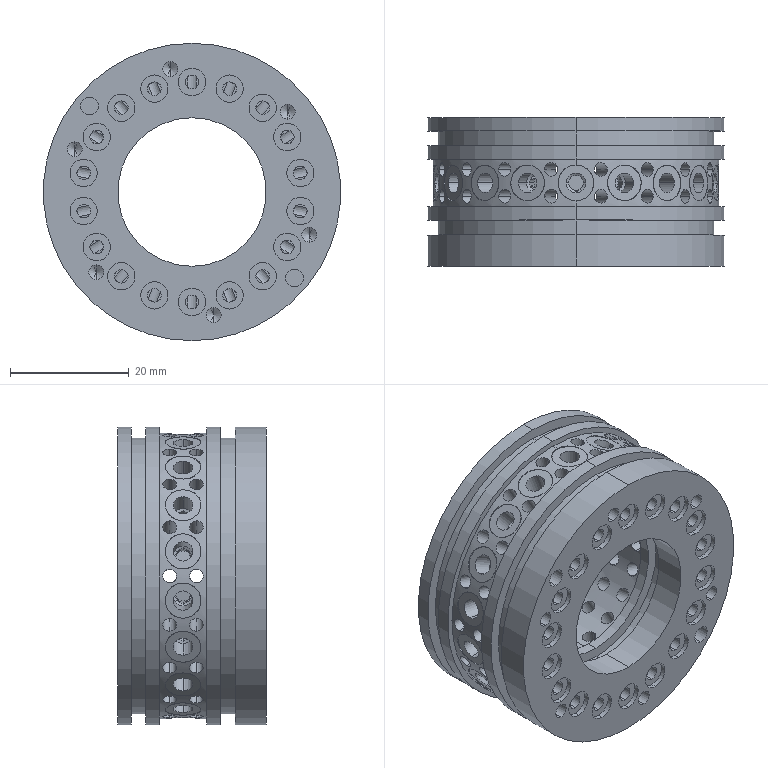Part | SolidWorks | features ICE 10, CirPattern 7, RevCut 4, 3DProfileFeature 3, HoleWzd 3, Extrusion 1 | 1 solid | 518 faces | box 50 x 25 x 50 mm | volume 28729 mm3 | cylinder 352 | plane 106 | cone 60 | commonest cylinder face diameters 2.3 x152 2.5 x60 3.3 x36 4.6 x36 6 x36 25 x8